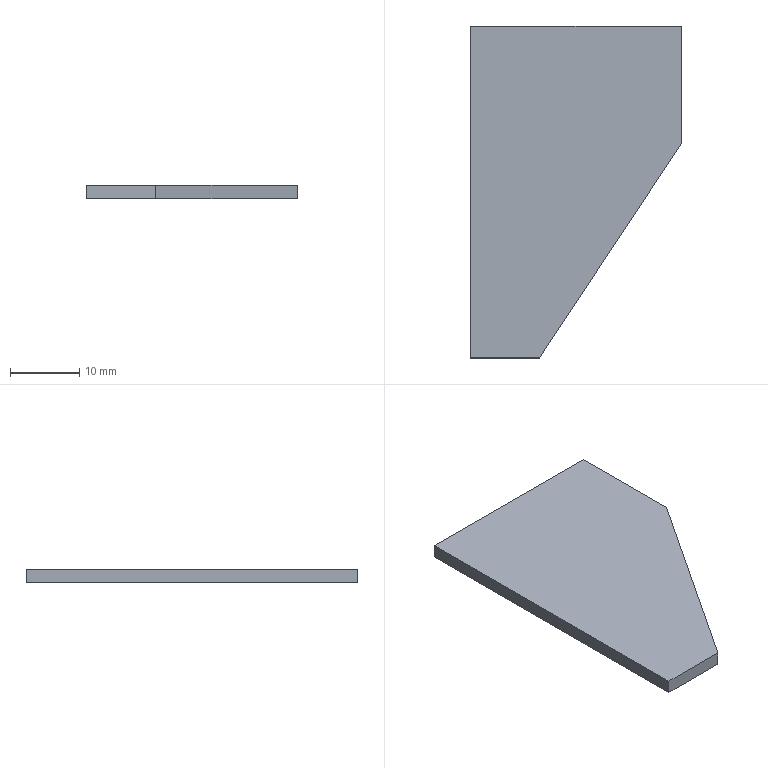Part | SolidWorks | features Extrusion 1 | 1 solid | 7 faces | box 30.5 x 48 x 2 mm | volume 2292 mm3 | plane 7
STEP:
#1=CARTESIAN_POINT('',(0.,0.,0.));
#2=VERTEX_POINT('',#1);
#3=CARTESIAN_POINT('',(0.,-48.,0.));
#4=VERTEX_POINT('',#3);
#5=CARTESIAN_POINT('',(0.,-48.,0.));
#6=DIRECTION('',(0.,-1.,0.));
#7=VECTOR('',#6,1000.);
#8=LINE('',#5,#7);
#9=EDGE_CURVE('',#2,#4,#8,.T.);
#10=ORIENTED_EDGE('',*,*,#9,.T.);
#11=CARTESIAN_POINT('',(0.,-48.,2.));
#12=VERTEX_POINT('',#11);
#13=CARTESIAN_POINT('',(0.,-48.,2.));
#14=DIRECTION('',(0.,0.,-1.));
#15=VECTOR('',#14,1000.);
#16=LINE('',#13,#15);
#17=EDGE_CURVE('',#12,#4,#16,.T.);
#18=ORIENTED_EDGE('',*,*,#17,.F.);
#19=CARTESIAN_POINT('',(0.,0.,2.));
#20=VERTEX_POINT('',#19);
#21=CARTESIAN_POINT('',(0.,-48.,2.));
#22=DIRECTION('',(0.,-1.,0.));
#23=VECTOR('',#22,1000.);
#24=LINE('',#21,#23);
#25=EDGE_CURVE('',#20,#12,#24,.T.);
#26=ORIENTED_EDGE('',*,*,#25,.F.);
#27=CARTESIAN_POINT('',(0.,0.,2.));
#28=DIRECTION('',(0.,0.,-1.));
#29=VECTOR('',#28,1000.);
#30=LINE('',#27,#29);
#31=EDGE_CURVE('',#20,#2,#30,.T.);
#32=ORIENTED_EDGE('',*,*,#31,.T.);
#33=EDGE_LOOP('',(#10,#18,#26,#32));
#34=FACE_OUTER_BOUND('',#33,.T.);
#35=CARTESIAN_POINT('',(0.,-48.,2.));
#36=DIRECTION('',(1.,0.,0.));
#37=DIRECTION('',(0.,0.,-1.));
#38=AXIS2_PLACEMENT_3D('',#35,#36,#37);
#39=PLANE('',#38);
#40=ADVANCED_FACE('',(#34),#39,.F.);
#41=CARTESIAN_POINT('',(10.,-48.,0.));
#42=VERTEX_POINT('',#41);
#43=CARTESIAN_POINT('',(10.,-48.,0.));
#44=DIRECTION('',(1.,0.,0.));
#45=VECTOR('',#44,1000.);
#46=LINE('',#43,#45);
#47=EDGE_CURVE('',#4,#42,#46,.T.);
#48=ORIENTED_EDGE('',*,*,#47,.T.);
#49=CARTESIAN_POINT('',(10.,-48.,2.));
#50=VERTEX_POINT('',#49);
#51=CARTESIAN_POINT('',(10.,-48.,2.));
#52=DIRECTION('',(0.,0.,-1.));
#53=VECTOR('',#52,1000.);
#54=LINE('',#51,#53);
#55=EDGE_CURVE('',#50,#42,#54,.T.);
#56=ORIENTED_EDGE('',*,*,#55,.F.);
#57=CARTESIAN_POINT('',(10.,-48.,2.));
#58=DIRECTION('',(1.,0.,0.));
#59=VECTOR('',#58,1000.);
#60=LINE('',#57,#59);
#61=EDGE_CURVE('',#12,#50,#60,.T.);
#62=ORIENTED_EDGE('',*,*,#61,.F.);
#63=ORIENTED_EDGE('',*,*,#17,.T.);
#64=EDGE_LOOP('',(#48,#56,#62,#63));
#65=FACE_OUTER_BOUND('',#64,.T.);
#66=CARTESIAN_POINT('',(10.,-48.,2.));
#67=DIRECTION('',(0.,1.,0.));
#68=DIRECTION('',(0.,0.,1.));
#69=AXIS2_PLACEMENT_3D('',#66,#67,#68);
#70=PLANE('',#69);
#71=ADVANCED_FACE('',(#65),#70,.F.);
#72=CARTESIAN_POINT('',(30.5,-17.,0.));
#73=VERTEX_POINT('',#72);
#74=CARTESIAN_POINT('',(30.5,-17.,0.));
#75=DIRECTION('',(0.5516,0.8341,0.));
#76=VECTOR('',#75,1000.);
#77=LINE('',#74,#76);
#78=EDGE_CURVE('',#42,#73,#77,.T.);
#79=ORIENTED_EDGE('',*,*,#78,.T.);
#80=CARTESIAN_POINT('',(30.5,-17.,2.));
#81=VERTEX_POINT('',#80);
#82=CARTESIAN_POINT('',(30.5,-17.,2.));
#83=DIRECTION('',(0.,0.,-1.));
#84=VECTOR('',#83,1000.);
#85=LINE('',#82,#84);
#86=EDGE_CURVE('',#81,#73,#85,.T.);
#87=ORIENTED_EDGE('',*,*,#86,.F.);
#88=CARTESIAN_POINT('',(30.5,-17.,2.));
#89=DIRECTION('',(0.5516,0.8341,0.));
#90=VECTOR('',#89,1000.);
#91=LINE('',#88,#90);
#92=EDGE_CURVE('',#50,#81,#91,.T.);
#93=ORIENTED_EDGE('',*,*,#92,.F.);
#94=ORIENTED_EDGE('',*,*,#55,.T.);
#95=EDGE_LOOP('',(#79,#87,#93,#94));
#96=FACE_OUTER_BOUND('',#95,.T.);
#97=CARTESIAN_POINT('',(30.5,-17.,2.));
#98=DIRECTION('',(-0.8341,0.5516,0.));
#99=DIRECTION('',(-0.5516,-0.8341,0.));
#100=AXIS2_PLACEMENT_3D('',#97,#98,#99);
#101=PLANE('',#100);
#102=ADVANCED_FACE('',(#96),#101,.F.);
#103=CARTESIAN_POINT('',(30.5,0.,0.));
#104=VERTEX_POINT('',#103);
#105=CARTESIAN_POINT('',(30.5,0.,0.));
#106=DIRECTION('',(0.,1.,0.));
#107=VECTOR('',#106,1000.);
#108=LINE('',#105,#107);
#109=EDGE_CURVE('',#73,#104,#108,.T.);
#110=ORIENTED_EDGE('',*,*,#109,.T.);
#111=CARTESIAN_POINT('',(30.5,0.,2.));
#112=VERTEX_POINT('',#111);
#113=CARTESIAN_POINT('',(30.5,0.,2.));
#114=DIRECTION('',(0.,0.,-1.));
#115=VECTOR('',#114,1000.);
#116=LINE('',#113,#115);
#117=EDGE_CURVE('',#112,#104,#116,.T.);
#118=ORIENTED_EDGE('',*,*,#117,.F.);
#119=CARTESIAN_POINT('',(30.5,0.,2.));
#120=DIRECTION('',(0.,1.,0.));
#121=VECTOR('',#120,1000.);
#122=LINE('',#119,#121);
#123=EDGE_CURVE('',#81,#112,#122,.T.);
#124=ORIENTED_EDGE('',*,*,#123,.F.);
#125=ORIENTED_EDGE('',*,*,#86,.T.);
#126=EDGE_LOOP('',(#110,#118,#124,#125));
#127=FACE_OUTER_BOUND('',#126,.T.);
#128=CARTESIAN_POINT('',(30.5,0.,2.));
#129=DIRECTION('',(-1.,0.,0.));
#130=DIRECTION('',(0.,-1.,0.));
#131=AXIS2_PLACEMENT_3D('',#128,#129,#130);
#132=PLANE('',#131);
#133=ADVANCED_FACE('',(#127),#132,.F.);
#134=CARTESIAN_POINT('',(0.,0.,0.));
#135=DIRECTION('',(-1.,0.,0.));
#136=VECTOR('',#135,1000.);
#137=LINE('',#134,#136);
#138=EDGE_CURVE('',#104,#2,#137,.T.);
#139=ORIENTED_EDGE('',*,*,#138,.T.);
#140=ORIENTED_EDGE('',*,*,#31,.F.);
#141=CARTESIAN_POINT('',(0.,0.,2.));
#142=DIRECTION('',(-1.,0.,0.));
#143=VECTOR('',#142,1000.);
#144=LINE('',#141,#143);
#145=EDGE_CURVE('',#112,#20,#144,.T.);
#146=ORIENTED_EDGE('',*,*,#145,.F.);
#147=ORIENTED_EDGE('',*,*,#117,.T.);
#148=EDGE_LOOP('',(#139,#140,#146,#147));
#149=FACE_OUTER_BOUND('',#148,.T.);
#150=CARTESIAN_POINT('',(0.,0.,2.));
#151=DIRECTION('',(0.,-1.,0.));
#152=DIRECTION('',(0.,0.,-1.));
#153=AXIS2_PLACEMENT_3D('',#150,#151,#152);
#154=PLANE('',#153);
#155=ADVANCED_FACE('',(#149),#154,.F.);
#156=ORIENTED_EDGE('',*,*,#25,.T.);
#157=ORIENTED_EDGE('',*,*,#61,.T.);
#158=ORIENTED_EDGE('',*,*,#92,.T.);
#159=ORIENTED_EDGE('',*,*,#123,.T.);
#160=ORIENTED_EDGE('',*,*,#145,.T.);
#161=EDGE_LOOP('',(#156,#157,#158,#159,#160));
#162=FACE_OUTER_BOUND('',#161,.T.);
#163=CARTESIAN_POINT('',(0.,0.,2.));
#164=DIRECTION('',(0.,0.,-1.));
#165=DIRECTION('',(-1.,0.,0.));
#166=AXIS2_PLACEMENT_3D('',#163,#164,#165);
#167=PLANE('',#166);
#168=ADVANCED_FACE('',(#162),#167,.F.);
#169=ORIENTED_EDGE('',*,*,#9,.F.);
#170=ORIENTED_EDGE('',*,*,#138,.F.);
#171=ORIENTED_EDGE('',*,*,#109,.F.);
#172=ORIENTED_EDGE('',*,*,#78,.F.);
#173=ORIENTED_EDGE('',*,*,#47,.F.);
#174=EDGE_LOOP('',(#169,#170,#171,#172,#173));
#175=FACE_OUTER_BOUND('',#174,.T.);
#176=CARTESIAN_POINT('',(0.,0.,0.));
#177=DIRECTION('',(0.,0.,-1.));
#178=DIRECTION('',(-1.,0.,0.));
#179=AXIS2_PLACEMENT_3D('',#176,#177,#178);
#180=PLANE('',#179);
#181=ADVANCED_FACE('',(#175),#180,.T.);
#182=CLOSED_SHELL('',(#40,#71,#102,#133,#155,#168,#181));
#183=MANIFOLD_SOLID_BREP('',#182);
#184=CARTESIAN_POINT('',(0.,0.,0.));
#185=DIRECTION('',(0.,0.,1.));
#186=DIRECTION('',(1.,0.,0.));
#187=AXIS2_PLACEMENT_3D('',#184,#185,#186);
#188=(LENGTH_UNIT()NAMED_UNIT(*)SI_UNIT(.MILLI.,.METRE.));
#189=UNCERTAINTY_MEASURE_WITH_UNIT(LENGTH_MEASURE(0.00001),#188,'','');
#190=(NAMED_UNIT(*)PLANE_ANGLE_UNIT()SI_UNIT($,.RADIAN.));
#191=(NAMED_UNIT(*)SI_UNIT($,.STERADIAN.)SOLID_ANGLE_UNIT());
#192=(GEOMETRIC_REPRESENTATION_CONTEXT(3)GLOBAL_UNCERTAINTY_ASSIGNED_CONTEXT((#189))GLOBAL_UNIT_ASSIGNED_CONTEXT((#188,#190,#191))REPRESENTATION_CONTEXT('',''));
#193=ADVANCED_BREP_SHAPE_REPRESENTATION('',(#183,#187),#192);